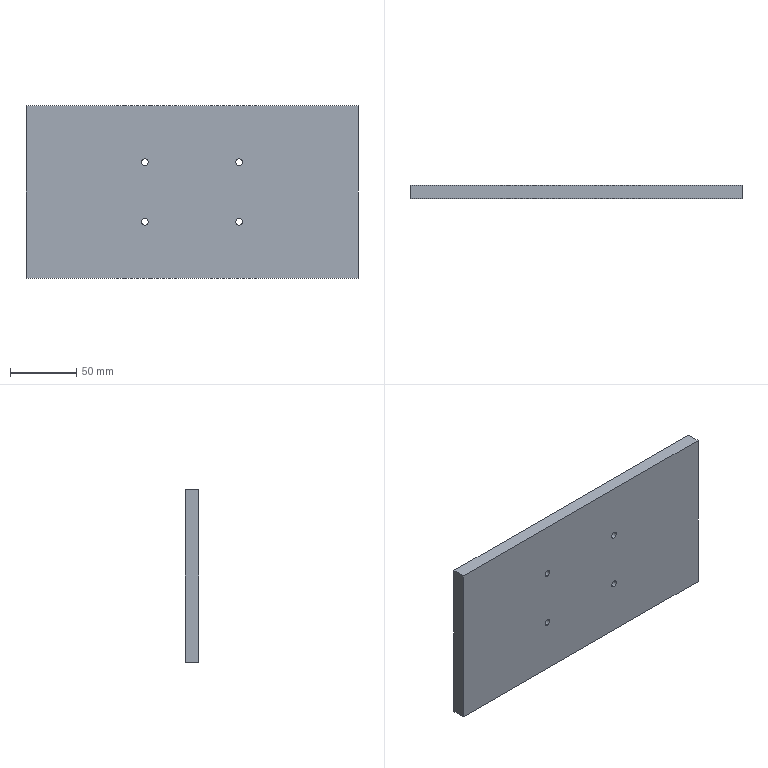Part | STEP file | A14-033 | 1 solid | 22 faces | box 250 x 10 x 130 mm | volume 324205 mm3 | cone 8 | cylinder 8 | plane 6 | commonest cylinder face diameters 5 x8
STEP:
#1=CARTESIAN_POINT('',(0.,0.,0.));
#2=DIRECTION('',(0.,0.,1.));
#3=DIRECTION('',(1.,0.,0.));
#4=AXIS2_PLACEMENT_3D('',#1,#2,#3);
#5=CARTESIAN_POINT('',(35.5,4.475,25.));
#6=VERTEX_POINT('',#5);
#7=CARTESIAN_POINT('',(35.5,5.,25.525));
#8=VERTEX_POINT('',#7);
#9=CARTESIAN_POINT('',(35.5,5.,25.525));
#10=DIRECTION('',(0.,0.7071,0.7071));
#11=VECTOR('',#10,1.);
#12=LINE('',#9,#11);
#13=CARTESIAN_POINT('',(35.5,5.,22.5));
#14=DIRECTION('',(0.,1.,0.));
#15=DIRECTION('',(0.,0.,1.));
#16=AXIS2_PLACEMENT_3D('',#13,#14,#15);
#17=CONICAL_SURFACE('',#16,3.025,0.7854);
#18=CARTESIAN_POINT('',(6.283,0.));
#19=DIRECTION('',(0.,1.));
#20=VECTOR('',#19,1.);
#21=LINE('',#18,#20);
#22=(GEOMETRIC_REPRESENTATION_CONTEXT(2)PARAMETRIC_REPRESENTATION_CONTEXT()REPRESENTATION_CONTEXT('',''));
#23=DEFINITIONAL_REPRESENTATION('',(#21),#22);
#24=PCURVE('',#17,#23);
#25=CARTESIAN_POINT('',(35.5,5.,22.5));
#26=DIRECTION('',(0.,1.,0.));
#27=DIRECTION('',(0.,0.,1.));
#28=AXIS2_PLACEMENT_3D('',#25,#26,#27);
#29=CONICAL_SURFACE('',#28,3.025,0.7854);
#30=CARTESIAN_POINT('',(0.,0.));
#31=DIRECTION('',(0.,1.));
#32=VECTOR('',#31,1.);
#33=LINE('',#30,#32);
#34=(GEOMETRIC_REPRESENTATION_CONTEXT(2)PARAMETRIC_REPRESENTATION_CONTEXT()REPRESENTATION_CONTEXT('',''));
#35=DEFINITIONAL_REPRESENTATION('',(#33),#34);
#36=PCURVE('',#29,#35);
#37=SURFACE_CURVE('',#12,(#24,#36),.PCURVE_S1.);
#38=EDGE_CURVE('',#6,#8,#37,.T.);
#39=ORIENTED_EDGE('',*,*,#38,.T.);
#40=CARTESIAN_POINT('',(35.5,5.,19.475));
#41=VERTEX_POINT('',#40);
#42=CARTESIAN_POINT('',(35.5,5.,22.5));
#43=DIRECTION('',(0.,1.,0.));
#44=DIRECTION('',(0.,0.,1.));
#45=AXIS2_PLACEMENT_3D('',#42,#43,#44);
#46=CIRCLE('',#45,3.025);
#47=CARTESIAN_POINT('',(0.,0.));
#48=DIRECTION('',(1.,0.));
#49=VECTOR('',#48,1.);
#50=LINE('',#47,#49);
#51=(GEOMETRIC_REPRESENTATION_CONTEXT(2)PARAMETRIC_REPRESENTATION_CONTEXT()REPRESENTATION_CONTEXT('',''));
#52=DEFINITIONAL_REPRESENTATION('',(#50),#51);
#53=PCURVE('',#17,#52);
#54=CARTESIAN_POINT('',(0.,5.,0.));
#55=DIRECTION('',(0.,1.,0.));
#56=DIRECTION('',(0.,0.,1.));
#57=AXIS2_PLACEMENT_3D('',#54,#55,#56);
#58=PLANE('',#57);
#59=CARTESIAN_POINT('',(22.5,35.5));
#60=DIRECTION('',(1.,0.));
#61=AXIS2_PLACEMENT_2D('',#59,#60);
#62=CIRCLE('',#61,3.025);
#63=(GEOMETRIC_REPRESENTATION_CONTEXT(2)PARAMETRIC_REPRESENTATION_CONTEXT()REPRESENTATION_CONTEXT('',''));
#64=DEFINITIONAL_REPRESENTATION('',(#62),#63);
#65=PCURVE('',#58,#64);
#66=SURFACE_CURVE('',#46,(#53,#65),.PCURVE_S1.);
#67=EDGE_CURVE('',#41,#8,#66,.T.);
#68=ORIENTED_EDGE('',*,*,#67,.F.);
#69=CARTESIAN_POINT('',(35.5,4.475,20.));
#70=VERTEX_POINT('',#69);
#71=CARTESIAN_POINT('',(35.5,5.,19.475));
#72=DIRECTION('',(0.,0.7071,-0.7071));
#73=VECTOR('',#72,1.);
#74=LINE('',#71,#73);
#75=CARTESIAN_POINT('',(3.142,0.));
#76=DIRECTION('',(0.,1.));
#77=VECTOR('',#76,1.);
#78=LINE('',#75,#77);
#79=(GEOMETRIC_REPRESENTATION_CONTEXT(2)PARAMETRIC_REPRESENTATION_CONTEXT()REPRESENTATION_CONTEXT('',''));
#80=DEFINITIONAL_REPRESENTATION('',(#78),#79);
#81=PCURVE('',#17,#80);
#82=CARTESIAN_POINT('',(3.142,0.));
#83=DIRECTION('',(0.,1.));
#84=VECTOR('',#83,1.);
#85=LINE('',#82,#84);
#86=(GEOMETRIC_REPRESENTATION_CONTEXT(2)PARAMETRIC_REPRESENTATION_CONTEXT()REPRESENTATION_CONTEXT('',''));
#87=DEFINITIONAL_REPRESENTATION('',(#85),#86);
#88=PCURVE('',#29,#87);
#89=SURFACE_CURVE('',#74,(#81,#88),.PCURVE_S1.);
#90=EDGE_CURVE('',#70,#41,#89,.T.);
#91=ORIENTED_EDGE('',*,*,#90,.F.);
#92=CARTESIAN_POINT('',(35.5,4.475,22.5));
#93=DIRECTION('',(0.,1.,0.));
#94=DIRECTION('',(0.,0.,1.));
#95=AXIS2_PLACEMENT_3D('',#92,#93,#94);
#96=CIRCLE('',#95,2.5);
#97=CARTESIAN_POINT('',(0.,-0.525));
#98=DIRECTION('',(1.,0.));
#99=VECTOR('',#98,1.);
#100=LINE('',#97,#99);
#101=(GEOMETRIC_REPRESENTATION_CONTEXT(2)PARAMETRIC_REPRESENTATION_CONTEXT()REPRESENTATION_CONTEXT('',''));
#102=DEFINITIONAL_REPRESENTATION('',(#100),#101);
#103=PCURVE('',#17,#102);
#104=CARTESIAN_POINT('',(35.5,5.,22.5));
#105=DIRECTION('',(0.,1.,0.));
#106=DIRECTION('',(0.,0.,1.));
#107=AXIS2_PLACEMENT_3D('',#104,#105,#106);
#108=CYLINDRICAL_SURFACE('',#107,2.5);
#109=CARTESIAN_POINT('',(0.,-0.525));
#110=DIRECTION('',(1.,0.));
#111=VECTOR('',#110,1.);
#112=LINE('',#109,#111);
#113=(GEOMETRIC_REPRESENTATION_CONTEXT(2)PARAMETRIC_REPRESENTATION_CONTEXT()REPRESENTATION_CONTEXT('',''));
#114=DEFINITIONAL_REPRESENTATION('',(#112),#113);
#115=PCURVE('',#108,#114);
#116=SURFACE_CURVE('',#96,(#103,#115),.PCURVE_S1.);
#117=EDGE_CURVE('',#70,#6,#116,.T.);
#118=ORIENTED_EDGE('',*,*,#117,.T.);
#119=EDGE_LOOP('',(#39,#68,#91,#118));
#120=FACE_BOUND('',#119,.F.);
#121=ADVANCED_FACE('',(#120),#17,.F.);
#122=CARTESIAN_POINT('',(35.5,-5.,25.));
#123=VERTEX_POINT('',#122);
#124=CARTESIAN_POINT('',(35.5,5.,25.));
#125=DIRECTION('',(0.,1.,0.));
#126=VECTOR('',#125,1.);
#127=LINE('',#124,#126);
#128=CARTESIAN_POINT('',(6.283,0.));
#129=DIRECTION('',(0.,1.));
#130=VECTOR('',#129,1.);
#131=LINE('',#128,#130);
#132=(GEOMETRIC_REPRESENTATION_CONTEXT(2)PARAMETRIC_REPRESENTATION_CONTEXT()REPRESENTATION_CONTEXT('',''));
#133=DEFINITIONAL_REPRESENTATION('',(#131),#132);
#134=PCURVE('',#108,#133);
#135=CARTESIAN_POINT('',(35.5,5.,22.5));
#136=DIRECTION('',(0.,1.,0.));
#137=DIRECTION('',(0.,0.,1.));
#138=AXIS2_PLACEMENT_3D('',#135,#136,#137);
#139=CYLINDRICAL_SURFACE('',#138,2.5);
#140=CARTESIAN_POINT('',(0.,0.));
#141=DIRECTION('',(0.,1.));
#142=VECTOR('',#141,1.);
#143=LINE('',#140,#142);
#144=(GEOMETRIC_REPRESENTATION_CONTEXT(2)PARAMETRIC_REPRESENTATION_CONTEXT()REPRESENTATION_CONTEXT('',''));
#145=DEFINITIONAL_REPRESENTATION('',(#143),#144);
#146=PCURVE('',#139,#145);
#147=SURFACE_CURVE('',#127,(#134,#146),.PCURVE_S1.);
#148=EDGE_CURVE('',#123,#6,#147,.T.);
#149=ORIENTED_EDGE('',*,*,#148,.T.);
#150=ORIENTED_EDGE('',*,*,#117,.F.);
#151=CARTESIAN_POINT('',(35.5,-5.,20.));
#152=VERTEX_POINT('',#151);
#153=CARTESIAN_POINT('',(35.5,5.,20.));
#154=DIRECTION('',(0.,1.,0.));
#155=VECTOR('',#154,1.);
#156=LINE('',#153,#155);
#157=CARTESIAN_POINT('',(3.142,0.));
#158=DIRECTION('',(0.,1.));
#159=VECTOR('',#158,1.);
#160=LINE('',#157,#159);
#161=(GEOMETRIC_REPRESENTATION_CONTEXT(2)PARAMETRIC_REPRESENTATION_CONTEXT()REPRESENTATION_CONTEXT('',''));
#162=DEFINITIONAL_REPRESENTATION('',(#160),#161);
#163=PCURVE('',#108,#162);
#164=CARTESIAN_POINT('',(3.142,0.));
#165=DIRECTION('',(0.,1.));
#166=VECTOR('',#165,1.);
#167=LINE('',#164,#166);
#168=(GEOMETRIC_REPRESENTATION_CONTEXT(2)PARAMETRIC_REPRESENTATION_CONTEXT()REPRESENTATION_CONTEXT('',''));
#169=DEFINITIONAL_REPRESENTATION('',(#167),#168);
#170=PCURVE('',#139,#169);
#171=SURFACE_CURVE('',#156,(#163,#170),.PCURVE_S1.);
#172=EDGE_CURVE('',#152,#70,#171,.T.);
#173=ORIENTED_EDGE('',*,*,#172,.F.);
#174=CARTESIAN_POINT('',(35.5,-5.,22.5));
#175=DIRECTION('',(0.,1.,0.));
#176=DIRECTION('',(0.,0.,1.));
#177=AXIS2_PLACEMENT_3D('',#174,#175,#176);
#178=CIRCLE('',#177,2.5);
#179=CARTESIAN_POINT('',(0.,-10.));
#180=DIRECTION('',(1.,0.));
#181=VECTOR('',#180,1.);
#182=LINE('',#179,#181);
#183=(GEOMETRIC_REPRESENTATION_CONTEXT(2)PARAMETRIC_REPRESENTATION_CONTEXT()REPRESENTATION_CONTEXT('',''));
#184=DEFINITIONAL_REPRESENTATION('',(#182),#183);
#185=PCURVE('',#108,#184);
#186=CARTESIAN_POINT('',(0.,-5.,0.));
#187=DIRECTION('',(0.,1.,0.));
#188=DIRECTION('',(0.,0.,1.));
#189=AXIS2_PLACEMENT_3D('',#186,#187,#188);
#190=PLANE('',#189);
#191=CARTESIAN_POINT('',(22.5,35.5));
#192=DIRECTION('',(1.,0.));
#193=AXIS2_PLACEMENT_2D('',#191,#192);
#194=CIRCLE('',#193,2.5);
#195=(GEOMETRIC_REPRESENTATION_CONTEXT(2)PARAMETRIC_REPRESENTATION_CONTEXT()REPRESENTATION_CONTEXT('',''));
#196=DEFINITIONAL_REPRESENTATION('',(#194),#195);
#197=PCURVE('',#190,#196);
#198=SURFACE_CURVE('',#178,(#185,#197),.PCURVE_S1.);
#199=EDGE_CURVE('',#152,#123,#198,.T.);
#200=ORIENTED_EDGE('',*,*,#199,.T.);
#201=EDGE_LOOP('',(#149,#150,#173,#200));
#202=FACE_BOUND('',#201,.F.);
#203=ADVANCED_FACE('',(#202),#108,.F.);
#204=CARTESIAN_POINT('',(35.5,4.475,-20.));
#205=VERTEX_POINT('',#204);
#206=CARTESIAN_POINT('',(35.5,5.,-19.475));
#207=VERTEX_POINT('',#206);
#208=CARTESIAN_POINT('',(35.5,5.,-19.475));
#209=DIRECTION('',(0.,0.7071,0.7071));
#210=VECTOR('',#209,1.);
#211=LINE('',#208,#210);
#212=CARTESIAN_POINT('',(35.5,5.,-22.5));
#213=DIRECTION('',(0.,1.,0.));
#214=DIRECTION('',(0.,0.,1.));
#215=AXIS2_PLACEMENT_3D('',#212,#213,#214);
#216=CONICAL_SURFACE('',#215,3.025,0.7854);
#217=CARTESIAN_POINT('',(6.283,0.));
#218=DIRECTION('',(0.,1.));
#219=VECTOR('',#218,1.);
#220=LINE('',#217,#219);
#221=(GEOMETRIC_REPRESENTATION_CONTEXT(2)PARAMETRIC_REPRESENTATION_CONTEXT()REPRESENTATION_CONTEXT('',''));
#222=DEFINITIONAL_REPRESENTATION('',(#220),#221);
#223=PCURVE('',#216,#222);
#224=CARTESIAN_POINT('',(35.5,5.,-22.5));
#225=DIRECTION('',(0.,1.,0.));
#226=DIRECTION('',(0.,0.,1.));
#227=AXIS2_PLACEMENT_3D('',#224,#225,#226);
#228=CONICAL_SURFACE('',#227,3.025,0.7854);
#229=CARTESIAN_POINT('',(0.,0.));
#230=DIRECTION('',(0.,1.));
#231=VECTOR('',#230,1.);
#232=LINE('',#229,#231);
#233=(GEOMETRIC_REPRESENTATION_CONTEXT(2)PARAMETRIC_REPRESENTATION_CONTEXT()REPRESENTATION_CONTEXT('',''));
#234=DEFINITIONAL_REPRESENTATION('',(#232),#233);
#235=PCURVE('',#228,#234);
#236=SURFACE_CURVE('',#211,(#223,#235),.PCURVE_S1.);
#237=EDGE_CURVE('',#205,#207,#236,.T.);
#238=ORIENTED_EDGE('',*,*,#237,.T.);
#239=CARTESIAN_POINT('',(35.5,5.,-25.525));
#240=VERTEX_POINT('',#239);
#241=CARTESIAN_POINT('',(35.5,5.,-22.5));
#242=DIRECTION('',(0.,1.,0.));
#243=DIRECTION('',(0.,0.,1.));
#244=AXIS2_PLACEMENT_3D('',#241,#242,#243);
#245=CIRCLE('',#244,3.025);
#246=CARTESIAN_POINT('',(0.,0.));
#247=DIRECTION('',(1.,0.));
#248=VECTOR('',#247,1.);
#249=LINE('',#246,#248);
#250=(GEOMETRIC_REPRESENTATION_CONTEXT(2)PARAMETRIC_REPRESENTATION_CONTEXT()REPRESENTATION_CONTEXT('',''));
#251=DEFINITIONAL_REPRESENTATION('',(#249),#250);
#252=PCURVE('',#216,#251);
#253=CARTESIAN_POINT('',(-22.5,35.5));
#254=DIRECTION('',(1.,0.));
#255=AXIS2_PLACEMENT_2D('',#253,#254);
#256=CIRCLE('',#255,3.025);
#257=(GEOMETRIC_REPRESENTATION_CONTEXT(2)PARAMETRIC_REPRESENTATION_CONTEXT()REPRESENTATION_CONTEXT('',''));
#258=DEFINITIONAL_REPRESENTATION('',(#256),#257);
#259=PCURVE('',#58,#258);
#260=SURFACE_CURVE('',#245,(#252,#259),.PCURVE_S1.);
#261=EDGE_CURVE('',#240,#207,#260,.T.);
#262=ORIENTED_EDGE('',*,*,#261,.F.);
#263=CARTESIAN_POINT('',(35.5,4.475,-25.));
#264=VERTEX_POINT('',#263);
#265=CARTESIAN_POINT('',(35.5,5.,-25.525));
#266=DIRECTION('',(0.,0.7071,-0.7071));
#267=VECTOR('',#266,1.);
#268=LINE('',#265,#267);
#269=CARTESIAN_POINT('',(3.142,0.));
#270=DIRECTION('',(0.,1.));
#271=VECTOR('',#270,1.);
#272=LINE('',#269,#271);
#273=(GEOMETRIC_REPRESENTATION_CONTEXT(2)PARAMETRIC_REPRESENTATION_CONTEXT()REPRESENTATION_CONTEXT('',''));
#274=DEFINITIONAL_REPRESENTATION('',(#272),#273);
#275=PCURVE('',#216,#274);
#276=CARTESIAN_POINT('',(3.142,0.));
#277=DIRECTION('',(0.,1.));
#278=VECTOR('',#277,1.);
#279=LINE('',#276,#278);
#280=(GEOMETRIC_REPRESENTATION_CONTEXT(2)PARAMETRIC_REPRESENTATION_CONTEXT()REPRESENTATION_CONTEXT('',''));
#281=DEFINITIONAL_REPRESENTATION('',(#279),#280);
#282=PCURVE('',#228,#281);
#283=SURFACE_CURVE('',#268,(#275,#282),.PCURVE_S1.);
#284=EDGE_CURVE('',#264,#240,#283,.T.);
#285=ORIENTED_EDGE('',*,*,#284,.F.);
#286=CARTESIAN_POINT('',(35.5,4.475,-22.5));
#287=DIRECTION('',(0.,1.,0.));
#288=DIRECTION('',(0.,0.,1.));
#289=AXIS2_PLACEMENT_3D('',#286,#287,#288);
#290=CIRCLE('',#289,2.5);
#291=CARTESIAN_POINT('',(0.,-0.525));
#292=DIRECTION('',(1.,0.));
#293=VECTOR('',#292,1.);
#294=LINE('',#291,#293);
#295=(GEOMETRIC_REPRESENTATION_CONTEXT(2)PARAMETRIC_REPRESENTATION_CONTEXT()REPRESENTATION_CONTEXT('',''));
#296=DEFINITIONAL_REPRESENTATION('',(#294),#295);
#297=PCURVE('',#216,#296);
#298=CARTESIAN_POINT('',(35.5,5.,-22.5));
#299=DIRECTION('',(0.,1.,0.));
#300=DIRECTION('',(0.,0.,1.));
#301=AXIS2_PLACEMENT_3D('',#298,#299,#300);
#302=CYLINDRICAL_SURFACE('',#301,2.5);
#303=CARTESIAN_POINT('',(0.,-0.525));
#304=DIRECTION('',(1.,0.));
#305=VECTOR('',#304,1.);
#306=LINE('',#303,#305);
#307=(GEOMETRIC_REPRESENTATION_CONTEXT(2)PARAMETRIC_REPRESENTATION_CONTEXT()REPRESENTATION_CONTEXT('',''));
#308=DEFINITIONAL_REPRESENTATION('',(#306),#307);
#309=PCURVE('',#302,#308);
#310=SURFACE_CURVE('',#290,(#297,#309),.PCURVE_S1.);
#311=EDGE_CURVE('',#264,#205,#310,.T.);
#312=ORIENTED_EDGE('',*,*,#311,.T.);
#313=EDGE_LOOP('',(#238,#262,#285,#312));
#314=FACE_BOUND('',#313,.F.);
#315=ADVANCED_FACE('',(#314),#216,.F.);
#316=CARTESIAN_POINT('',(35.5,-5.,-20.));
#317=VERTEX_POINT('',#316);
#318=CARTESIAN_POINT('',(35.5,5.,-20.));
#319=DIRECTION('',(0.,1.,0.));
#320=VECTOR('',#319,1.);
#321=LINE('',#318,#320);
#322=CARTESIAN_POINT('',(6.283,0.));
#323=DIRECTION('',(0.,1.));
#324=VECTOR('',#323,1.);
#325=LINE('',#322,#324);
#326=(GEOMETRIC_REPRESENTATION_CONTEXT(2)PARAMETRIC_REPRESENTATION_CONTEXT()REPRESENTATION_CONTEXT('',''));
#327=DEFINITIONAL_REPRESENTATION('',(#325),#326);
#328=PCURVE('',#302,#327);
#329=CARTESIAN_POINT('',(35.5,5.,-22.5));
#330=DIRECTION('',(0.,1.,0.));
#331=DIRECTION('',(0.,0.,1.));
#332=AXIS2_PLACEMENT_3D('',#329,#330,#331);
#333=CYLINDRICAL_SURFACE('',#332,2.5);
#334=CARTESIAN_POINT('',(0.,0.));
#335=DIRECTION('',(0.,1.));
#336=VECTOR('',#335,1.);
#337=LINE('',#334,#336);
#338=(GEOMETRIC_REPRESENTATION_CONTEXT(2)PARAMETRIC_REPRESENTATION_CONTEXT()REPRESENTATION_CONTEXT('',''));
#339=DEFINITIONAL_REPRESENTATION('',(#337),#338);
#340=PCURVE('',#333,#339);
#341=SURFACE_CURVE('',#321,(#328,#340),.PCURVE_S1.);
#342=EDGE_CURVE('',#317,#205,#341,.T.);
#343=ORIENTED_EDGE('',*,*,#342,.T.);
#344=ORIENTED_EDGE('',*,*,#311,.F.);
#345=CARTESIAN_POINT('',(35.5,-5.,-25.));
#346=VERTEX_POINT('',#345);
#347=CARTESIAN_POINT('',(35.5,5.,-25.));
#348=DIRECTION('',(0.,1.,0.));
#349=VECTOR('',#348,1.);
#350=LINE('',#347,#349);
#351=CARTESIAN_POINT('',(3.142,0.));
#352=DIRECTION('',(0.,1.));
#353=VECTOR('',#352,1.);
#354=LINE('',#351,#353);
#355=(GEOMETRIC_REPRESENTATION_CONTEXT(2)PARAMETRIC_REPRESENTATION_CONTEXT()REPRESENTATION_CONTEXT('',''));
#356=DEFINITIONAL_REPRESENTATION('',(#354),#355);
#357=PCURVE('',#302,#356);
#358=CARTESIAN_POINT('',(3.142,0.));
#359=DIRECTION('',(0.,1.));
#360=VECTOR('',#359,1.);
#361=LINE('',#358,#360);
#362=(GEOMETRIC_REPRESENTATION_CONTEXT(2)PARAMETRIC_REPRESENTATION_CONTEXT()REPRESENTATION_CONTEXT('',''));
#363=DEFINITIONAL_REPRESENTATION('',(#361),#362);
#364=PCURVE('',#333,#363);
#365=SURFACE_CURVE('',#350,(#357,#364),.PCURVE_S1.);
#366=EDGE_CURVE('',#346,#264,#365,.T.);
#367=ORIENTED_EDGE('',*,*,#366,.F.);
#368=CARTESIAN_POINT('',(35.5,-5.,-22.5));
#369=DIRECTION('',(0.,1.,0.));
#370=DIRECTION('',(0.,0.,1.));
#371=AXIS2_PLACEMENT_3D('',#368,#369,#370);
#372=CIRCLE('',#371,2.5);
#373=CARTESIAN_POINT('',(0.,-10.));
#374=DIRECTION('',(1.,0.));
#375=VECTOR('',#374,1.);
#376=LINE('',#373,#375);
#377=(GEOMETRIC_REPRESENTATION_CONTEXT(2)PARAMETRIC_REPRESENTATION_CONTEXT()REPRESENTATION_CONTEXT('',''));
#378=DEFINITIONAL_REPRESENTATION('',(#376),#377);
#379=PCURVE('',#302,#378);
#380=CARTESIAN_POINT('',(-22.5,35.5));
#381=DIRECTION('',(1.,0.));
#382=AXIS2_PLACEMENT_2D('',#380,#381);
#383=CIRCLE('',#382,2.5);
#384=(GEOMETRIC_REPRESENTATION_CONTEXT(2)PARAMETRIC_REPRESENTATION_CONTEXT()REPRESENTATION_CONTEXT('',''));
#385=DEFINITIONAL_REPRESENTATION('',(#383),#384);
#386=PCURVE('',#190,#385);
#387=SURFACE_CURVE('',#372,(#379,#386),.PCURVE_S1.);
#388=EDGE_CURVE('',#346,#317,#387,.T.);
#389=ORIENTED_EDGE('',*,*,#388,.T.);
#390=EDGE_LOOP('',(#343,#344,#367,#389));
#391=FACE_BOUND('',#390,.F.);
#392=ADVANCED_FACE('',(#391),#302,.F.);
#393=CARTESIAN_POINT('',(-35.5,4.475,25.));
#394=VERTEX_POINT('',#393);
#395=CARTESIAN_POINT('',(-35.5,5.,25.525));
#396=VERTEX_POINT('',#395);
#397=CARTESIAN_POINT('',(-35.5,5.,25.525));
#398=DIRECTION('',(0.,0.7071,0.7071));
#399=VECTOR('',#398,1.);
#400=LINE('',#397,#399);
#401=CARTESIAN_POINT('',(-35.5,5.,22.5));
#402=DIRECTION('',(0.,1.,0.));
#403=DIRECTION('',(0.,0.,1.));
#404=AXIS2_PLACEMENT_3D('',#401,#402,#403);
#405=CONICAL_SURFACE('',#404,3.025,0.7854);
#406=CARTESIAN_POINT('',(6.283,0.));
#407=DIRECTION('',(0.,1.));
#408=VECTOR('',#407,1.);
#409=LINE('',#406,#408);
#410=(GEOMETRIC_REPRESENTATION_CONTEXT(2)PARAMETRIC_REPRESENTATION_CONTEXT()REPRESENTATION_CONTEXT('',''));
#411=DEFINITIONAL_REPRESENTATION('',(#409),#410);
#412=PCURVE('',#405,#411);
#413=CARTESIAN_POINT('',(-35.5,5.,22.5));
#414=DIRECTION('',(0.,1.,0.));
#415=DIRECTION('',(0.,0.,1.));
#416=AXIS2_PLACEMENT_3D('',#413,#414,#415);
#417=CONICAL_SURFACE('',#416,3.025,0.7854);
#418=CARTESIAN_POINT('',(0.,0.));
#419=DIRECTION('',(0.,1.));
#420=VECTOR('',#419,1.);
#421=LINE('',#418,#420);
#422=(GEOMETRIC_REPRESENTATION_CONTEXT(2)PARAMETRIC_REPRESENTATION_CONTEXT()REPRESENTATION_CONTEXT('',''));
#423=DEFINITIONAL_REPRESENTATION('',(#421),#422);
#424=PCURVE('',#417,#423);
#425=SURFACE_CURVE('',#400,(#412,#424),.PCURVE_S1.);
#426=EDGE_CURVE('',#394,#396,#425,.T.);
#427=ORIENTED_EDGE('',*,*,#426,.T.);
#428=CARTESIAN_POINT('',(-35.5,5.,19.475));
#429=VERTEX_POINT('',#428);
#430=CARTESIAN_POINT('',(-35.5,5.,22.5));
#431=DIRECTION('',(0.,1.,0.));
#432=DIRECTION('',(0.,0.,1.));
#433=AXIS2_PLACEMENT_3D('',#430,#431,#432);
#434=CIRCLE('',#433,3.025);
#435=CARTESIAN_POINT('',(0.,0.));
#436=DIRECTION('',(1.,0.));
#437=VECTOR('',#436,1.);
#438=LINE('',#435,#437);
#439=(GEOMETRIC_REPRESENTATION_CONTEXT(2)PARAMETRIC_REPRESENTATION_CONTEXT()REPRESENTATION_CONTEXT('',''));
#440=DEFINITIONAL_REPRESENTATION('',(#438),#439);
#441=PCURVE('',#405,#440);
#442=CARTESIAN_POINT('',(22.5,-35.5));
#443=DIRECTION('',(1.,0.));
#444=AXIS2_PLACEMENT_2D('',#442,#443);
#445=CIRCLE('',#444,3.025);
#446=(GEOMETRIC_REPRESENTATION_CONTEXT(2)PARAMETRIC_REPRESENTATION_CONTEXT()REPRESENTATION_CONTEXT('',''));
#447=DEFINITIONAL_REPRESENTATION('',(#445),#446);
#448=PCURVE('',#58,#447);
#449=SURFACE_CURVE('',#434,(#441,#448),.PCURVE_S1.);
#450=EDGE_CURVE('',#429,#396,#449,.T.);
#451=ORIENTED_EDGE('',*,*,#450,.F.);
#452=CARTESIAN_POINT('',(-35.5,4.475,20.));
#453=VERTEX_POINT('',#452);
#454=CARTESIAN_POINT('',(-35.5,5.,19.475));
#455=DIRECTION('',(0.,0.7071,-0.7071));
#456=VECTOR('',#455,1.);
#457=LINE('',#454,#456);
#458=CARTESIAN_POINT('',(3.142,0.));
#459=DIRECTION('',(0.,1.));
#460=VECTOR('',#459,1.);
#461=LINE('',#458,#460);
#462=(GEOMETRIC_REPRESENTATION_CONTEXT(2)PARAMETRIC_REPRESENTATION_CONTEXT()REPRESENTATION_CONTEXT('',''));
#463=DEFINITIONAL_REPRESENTATION('',(#461),#462);
#464=PCURVE('',#405,#463);
#465=CARTESIAN_POINT('',(3.142,0.));
#466=DIRECTION('',(0.,1.));
#467=VECTOR('',#466,1.);
#468=LINE('',#465,#467);
#469=(GEOMETRIC_REPRESENTATION_CONTEXT(2)PARAMETRIC_REPRESENTATION_CONTEXT()REPRESENTATION_CONTEXT('',''));
#470=DEFINITIONAL_REPRESENTATION('',(#468),#469);
#471=PCURVE('',#417,#470);
#472=SURFACE_CURVE('',#457,(#464,#471),.PCURVE_S1.);
#473=EDGE_CURVE('',#453,#429,#472,.T.);
#474=ORIENTED_EDGE('',*,*,#473,.F.);
#475=CARTESIAN_POINT('',(-35.5,4.475,22.5));
#476=DIRECTION('',(0.,1.,0.));
#477=DIRECTION('',(0.,0.,1.));
#478=AXIS2_PLACEMENT_3D('',#475,#476,#477);
#479=CIRCLE('',#478,2.5);
#480=CARTESIAN_POINT('',(0.,-0.525));
#481=DIRECTION('',(1.,0.));
#482=VECTOR('',#481,1.);
#483=LINE('',#480,#482);
#484=(GEOMETRIC_REPRESENTATION_CONTEXT(2)PARAMETRIC_REPRESENTATION_CONTEXT()REPRESENTATION_CONTEXT('',''));
#485=DEFINITIONAL_REPRESENTATION('',(#483),#484);
#486=PCURVE('',#405,#485);
#487=CARTESIAN_POINT('',(-35.5,5.,22.5));
#488=DIRECTION('',(0.,1.,0.));
#489=DIRECTION('',(0.,0.,1.));
#490=AXIS2_PLACEMENT_3D('',#487,#488,#489);
#491=CYLINDRICAL_SURFACE('',#490,2.5);
#492=CARTESIAN_POINT('',(0.,-0.525));
#493=DIRECTION('',(1.,0.));
#494=VECTOR('',#493,1.);
#495=LINE('',#492,#494);
#496=(GEOMETRIC_REPRESENTATION_CONTEXT(2)PARAMETRIC_REPRESENTATION_CONTEXT()REPRESENTATION_CONTEXT('',''));
#497=DEFINITIONAL_REPRESENTATION('',(#495),#496);
#498=PCURVE('',#491,#497);
#499=SURFACE_CURVE('',#479,(#486,#498),.PCURVE_S1.);
#500=EDGE_CURVE('',#453,#394,#499,.T.);
#501=ORIENTED_EDGE('',*,*,#500,.T.);
#502=EDGE_LOOP('',(#427,#451,#474,#501));
#503=FACE_BOUND('',#502,.F.);
#504=ADVANCED_FACE('',(#503),#405,.F.);
#505=CARTESIAN_POINT('',(-35.5,-5.,25.));
#506=VERTEX_POINT('',#505);
#507=CARTESIAN_POINT('',(-35.5,5.,25.));
#508=DIRECTION('',(0.,1.,0.));
#509=VECTOR('',#508,1.);
#510=LINE('',#507,#509);
#511=CARTESIAN_POINT('',(6.283,0.));
#512=DIRECTION('',(0.,1.));
#513=VECTOR('',#512,1.);
#514=LINE('',#511,#513);
#515=(GEOMETRIC_REPRESENTATION_CONTEXT(2)PARAMETRIC_REPRESENTATION_CONTEXT()REPRESENTATION_CONTEXT('',''));
#516=DEFINITIONAL_REPRESENTATION('',(#514),#515);
#517=PCURVE('',#491,#516);
#518=CARTESIAN_POINT('',(-35.5,5.,22.5));
#519=DIRECTION('',(0.,1.,0.));
#520=DIRECTION('',(0.,0.,1.));
#521=AXIS2_PLACEMENT_3D('',#518,#519,#520);
#522=CYLINDRICAL_SURFACE('',#521,2.5);
#523=CARTESIAN_POINT('',(0.,0.));
#524=DIRECTION('',(0.,1.));
#525=VECTOR('',#524,1.);
#526=LINE('',#523,#525);
#527=(GEOMETRIC_REPRESENTATION_CONTEXT(2)PARAMETRIC_REPRESENTATION_CONTEXT()REPRESENTATION_CONTEXT('',''));
#528=DEFINITIONAL_REPRESENTATION('',(#526),#527);
#529=PCURVE('',#522,#528);
#530=SURFACE_CURVE('',#510,(#517,#529),.PCURVE_S1.);
#531=EDGE_CURVE('',#506,#394,#530,.T.);
#532=ORIENTED_EDGE('',*,*,#531,.T.);
#533=ORIENTED_EDGE('',*,*,#500,.F.);
#534=CARTESIAN_POINT('',(-35.5,-5.,20.));
#535=VERTEX_POINT('',#534);
#536=CARTESIAN_POINT('',(-35.5,5.,20.));
#537=DIRECTION('',(0.,1.,0.));
#538=VECTOR('',#537,1.);
#539=LINE('',#536,#538);
#540=CARTESIAN_POINT('',(3.142,0.));
#541=DIRECTION('',(0.,1.));
#542=VECTOR('',#541,1.);
#543=LINE('',#540,#542);
#544=(GEOMETRIC_REPRESENTATION_CONTEXT(2)PARAMETRIC_REPRESENTATION_CONTEXT()REPRESENTATION_CONTEXT('',''));
#545=DEFINITIONAL_REPRESENTATION('',(#543),#544);
#546=PCURVE('',#491,#545);
#547=CARTESIAN_POINT('',(3.142,0.));
#548=DIRECTION('',(0.,1.));
#549=VECTOR('',#548,1.);
#550=LINE('',#547,#549);
#551=(GEOMETRIC_REPRESENTATION_CONTEXT(2)PARAMETRIC_REPRESENTATION_CONTEXT()REPRESENTATION_CONTEXT('',''));
#552=DEFINITIONAL_REPRESENTATION('',(#550),#551);
#553=PCURVE('',#522,#552);
#554=SURFACE_CURVE('',#539,(#546,#553),.PCURVE_S1.);
#555=EDGE_CURVE('',#535,#453,#554,.T.);
#556=ORIENTED_EDGE('',*,*,#555,.F.);
#557=CARTESIAN_POINT('',(-35.5,-5.,22.5));
#558=DIRECTION('',(0.,1.,0.));
#559=DIRECTION('',(0.,0.,1.));
#560=AXIS2_PLACEMENT_3D('',#557,#558,#559);
#561=CIRCLE('',#560,2.5);
#562=CARTESIAN_POINT('',(0.,-10.));
#563=DIRECTION('',(1.,0.));
#564=VECTOR('',#563,1.);
#565=LINE('',#562,#564);
#566=(GEOMETRIC_REPRESENTATION_CONTEXT(2)PARAMETRIC_REPRESENTATION_CONTEXT()REPRESENTATION_CONTEXT('',''));
#567=DEFINITIONAL_REPRESENTATION('',(#565),#566);
#568=PCURVE('',#491,#567);
#569=CARTESIAN_POINT('',(22.5,-35.5));
#570=DIRECTION('',(1.,0.));
#571=AXIS2_PLACEMENT_2D('',#569,#570);
#572=CIRCLE('',#571,2.5);
#573=(GEOMETRIC_REPRESENTATION_CONTEXT(2)PARAMETRIC_REPRESENTATION_CONTEXT()REPRESENTATION_CONTEXT('',''));
#574=DEFINITIONAL_REPRESENTATION('',(#572),#573);
#575=PCURVE('',#190,#574);
#576=SURFACE_CURVE('',#561,(#568,#575),.PCURVE_S1.);
#577=EDGE_CURVE('',#535,#506,#576,.T.);
#578=ORIENTED_EDGE('',*,*,#577,.T.);
#579=EDGE_LOOP('',(#532,#533,#556,#578));
#580=FACE_BOUND('',#579,.F.);
#581=ADVANCED_FACE('',(#580),#491,.F.);
#582=CARTESIAN_POINT('',(-35.5,4.475,-20.));
#583=VERTEX_POINT('',#582);
#584=CARTESIAN_POINT('',(-35.5,5.,-19.475));
#585=VERTEX_POINT('',#584);
#586=CARTESIAN_POINT('',(-35.5,5.,-19.475));
#587=DIRECTION('',(0.,0.7071,0.7071));
#588=VECTOR('',#587,1.);
#589=LINE('',#586,#588);
#590=CARTESIAN_POINT('',(-35.5,5.,-22.5));
#591=DIRECTION('',(0.,1.,0.));
#592=DIRECTION('',(0.,0.,1.));
#593=AXIS2_PLACEMENT_3D('',#590,#591,#592);
#594=CONICAL_SURFACE('',#593,3.025,0.7854);
#595=CARTESIAN_POINT('',(6.283,0.));
#596=DIRECTION('',(0.,1.));
#597=VECTOR('',#596,1.);
#598=LINE('',#595,#597);
#599=(GEOMETRIC_REPRESENTATION_CONTEXT(2)PARAMETRIC_REPRESENTATION_CONTEXT()REPRESENTATION_CONTEXT('',''));
#600=DEFINITIONAL_REPRESENTATION('',(#598),#599);
#601=PCURVE('',#594,#600);
#602=CARTESIAN_POINT('',(-35.5,5.,-22.5));
#603=DIRECTION('',(0.,1.,0.));
#604=DIRECTION('',(0.,0.,1.));
#605=AXIS2_PLACEMENT_3D('',#602,#603,#604);
#606=CONICAL_SURFACE('',#605,3.025,0.7854);
#607=CARTESIAN_POINT('',(0.,0.));
#608=DIRECTION('',(0.,1.));
#609=VECTOR('',#608,1.);
#610=LINE('',#607,#609);
#611=(GEOMETRIC_REPRESENTATION_CONTEXT(2)PARAMETRIC_REPRESENTATION_CONTEXT()REPRESENTATION_CONTEXT('',''));
#612=DEFINITIONAL_REPRESENTATION('',(#610),#611);
#613=PCURVE('',#606,#612);
#614=SURFACE_CURVE('',#589,(#601,#613),.PCURVE_S1.);
#615=EDGE_CURVE('',#583,#585,#614,.T.);
#616=ORIENTED_EDGE('',*,*,#615,.T.);
#617=CARTESIAN_POINT('',(-35.5,5.,-25.525));
#618=VERTEX_POINT('',#617);
#619=CARTESIAN_POINT('',(-35.5,5.,-22.5));
#620=DIRECTION('',(0.,1.,0.));
#621=DIRECTION('',(0.,0.,1.));
#622=AXIS2_PLACEMENT_3D('',#619,#620,#621);
#623=CIRCLE('',#622,3.025);
#624=CARTESIAN_POINT('',(0.,0.));
#625=DIRECTION('',(1.,0.));
#626=VECTOR('',#625,1.);
#627=LINE('',#624,#626);
#628=(GEOMETRIC_REPRESENTATION_CONTEXT(2)PARAMETRIC_REPRESENTATION_CONTEXT()REPRESENTATION_CONTEXT('',''));
#629=DEFINITIONAL_REPRESENTATION('',(#627),#628);
#630=PCURVE('',#594,#629);
#631=CARTESIAN_POINT('',(-22.5,-35.5));
#632=DIRECTION('',(1.,0.));
#633=AXIS2_PLACEMENT_2D('',#631,#632);
#634=CIRCLE('',#633,3.025);
#635=(GEOMETRIC_REPRESENTATION_CONTEXT(2)PARAMETRIC_REPRESENTATION_CONTEXT()REPRESENTATION_CONTEXT('',''));
#636=DEFINITIONAL_REPRESENTATION('',(#634),#635);
#637=PCURVE('',#58,#636);
#638=SURFACE_CURVE('',#623,(#630,#637),.PCURVE_S1.);
#639=EDGE_CURVE('',#618,#585,#638,.T.);
#640=ORIENTED_EDGE('',*,*,#639,.F.);
#641=CARTESIAN_POINT('',(-35.5,4.475,-25.));
#642=VERTEX_POINT('',#641);
#643=CARTESIAN_POINT('',(-35.5,5.,-25.525));
#644=DIRECTION('',(0.,0.7071,-0.7071));
#645=VECTOR('',#644,1.);
#646=LINE('',#643,#645);
#647=CARTESIAN_POINT('',(3.142,0.));
#648=DIRECTION('',(0.,1.));
#649=VECTOR('',#648,1.);
#650=LINE('',#647,#649);
#651=(GEOMETRIC_REPRESENTATION_CONTEXT(2)PARAMETRIC_REPRESENTATION_CONTEXT()REPRESENTATION_CONTEXT('',''));
#652=DEFINITIONAL_REPRESENTATION('',(#650),#651);
#653=PCURVE('',#594,#652);
#654=CARTESIAN_POINT('',(3.142,0.));
#655=DIRECTION('',(0.,1.));
#656=VECTOR('',#655,1.);
#657=LINE('',#654,#656);
#658=(GEOMETRIC_REPRESENTATION_CONTEXT(2)PARAMETRIC_REPRESENTATION_CONTEXT()REPRESENTATION_CONTEXT('',''));
#659=DEFINITIONAL_REPRESENTATION('',(#657),#658);
#660=PCURVE('',#606,#659);
#661=SURFACE_CURVE('',#646,(#653,#660),.PCURVE_S1.);
#662=EDGE_CURVE('',#642,#618,#661,.T.);
#663=ORIENTED_EDGE('',*,*,#662,.F.);
#664=CARTESIAN_POINT('',(-35.5,4.475,-22.5));
#665=DIRECTION('',(0.,1.,0.));
#666=DIRECTION('',(0.,0.,1.));
#667=AXIS2_PLACEMENT_3D('',#664,#665,#666);
#668=CIRCLE('',#667,2.5);
#669=CARTESIAN_POINT('',(0.,-0.525));
#670=DIRECTION('',(1.,0.));
#671=VECTOR('',#670,1.);
#672=LINE('',#669,#671);
#673=(GEOMETRIC_REPRESENTATION_CONTEXT(2)PARAMETRIC_REPRESENTATION_CONTEXT()REPRESENTATION_CONTEXT('',''));
#674=DEFINITIONAL_REPRESENTATION('',(#672),#673);
#675=PCURVE('',#594,#674);
#676=CARTESIAN_POINT('',(-35.5,5.,-22.5));
#677=DIRECTION('',(0.,1.,0.));
#678=DIRECTION('',(0.,0.,1.));
#679=AXIS2_PLACEMENT_3D('',#676,#677,#678);
#680=CYLINDRICAL_SURFACE('',#679,2.5);
#681=CARTESIAN_POINT('',(0.,-0.525));
#682=DIRECTION('',(1.,0.));
#683=VECTOR('',#682,1.);
#684=LINE('',#681,#683);
#685=(GEOMETRIC_REPRESENTATION_CONTEXT(2)PARAMETRIC_REPRESENTATION_CONTEXT()REPRESENTATION_CONTEXT('',''));
#686=DEFINITIONAL_REPRESENTATION('',(#684),#685);
#687=PCURVE('',#680,#686);
#688=SURFACE_CURVE('',#668,(#675,#687),.PCURVE_S1.);
#689=EDGE_CURVE('',#642,#583,#688,.T.);
#690=ORIENTED_EDGE('',*,*,#689,.T.);
#691=EDGE_LOOP('',(#616,#640,#663,#690));
#692=FACE_BOUND('',#691,.F.);
#693=ADVANCED_FACE('',(#692),#594,.F.);
#694=CARTESIAN_POINT('',(-35.5,-5.,-20.));
#695=VERTEX_POINT('',#694);
#696=CARTESIAN_POINT('',(-35.5,5.,-20.));
#697=DIRECTION('',(0.,1.,0.));
#698=VECTOR('',#697,1.);
#699=LINE('',#696,#698);
#700=CARTESIAN_POINT('',(6.283,0.));
#701=DIRECTION('',(0.,1.));
#702=VECTOR('',#701,1.);
#703=LINE('',#700,#702);
#704=(GEOMETRIC_REPRESENTATION_CONTEXT(2)PARAMETRIC_REPRESENTATION_CONTEXT()REPRESENTATION_CONTEXT('',''));
#705=DEFINITIONAL_REPRESENTATION('',(#703),#704);
#706=PCURVE('',#680,#705);
#707=CARTESIAN_POINT('',(-35.5,5.,-22.5));
#708=DIRECTION('',(0.,1.,0.));
#709=DIRECTION('',(0.,0.,1.));
#710=AXIS2_PLACEMENT_3D('',#707,#708,#709);
#711=CYLINDRICAL_SURFACE('',#710,2.5);
#712=CARTESIAN_POINT('',(0.,0.));
#713=DIRECTION('',(0.,1.));
#714=VECTOR('',#713,1.);
#715=LINE('',#712,#714);
#716=(GEOMETRIC_REPRESENTATION_CONTEXT(2)PARAMETRIC_REPRESENTATION_CONTEXT()REPRESENTATION_CONTEXT('',''));
#717=DEFINITIONAL_REPRESENTATION('',(#715),#716);
#718=PCURVE('',#711,#717);
#719=SURFACE_CURVE('',#699,(#706,#718),.PCURVE_S1.);
#720=EDGE_CURVE('',#695,#583,#719,.T.);
#721=ORIENTED_EDGE('',*,*,#720,.T.);
#722=ORIENTED_EDGE('',*,*,#689,.F.);
#723=CARTESIAN_POINT('',(-35.5,-5.,-25.));
#724=VERTEX_POINT('',#723);
#725=CARTESIAN_POINT('',(-35.5,5.,-25.));
#726=DIRECTION('',(0.,1.,0.));
#727=VECTOR('',#726,1.);
#728=LINE('',#725,#727);
#729=CARTESIAN_POINT('',(3.142,0.));
#730=DIRECTION('',(0.,1.));
#731=VECTOR('',#730,1.);
#732=LINE('',#729,#731);
#733=(GEOMETRIC_REPRESENTATION_CONTEXT(2)PARAMETRIC_REPRESENTATION_CONTEXT()REPRESENTATION_CONTEXT('',''));
#734=DEFINITIONAL_REPRESENTATION('',(#732),#733);
#735=PCURVE('',#680,#734);
#736=CARTESIAN_POINT('',(3.142,0.));
#737=DIRECTION('',(0.,1.));
#738=VECTOR('',#737,1.);
#739=LINE('',#736,#738);
#740=(GEOMETRIC_REPRESENTATION_CONTEXT(2)PARAMETRIC_REPRESENTATION_CONTEXT()REPRESENTATION_CONTEXT('',''));
#741=DEFINITIONAL_REPRESENTATION('',(#739),#740);
#742=PCURVE('',#711,#741);
#743=SURFACE_CURVE('',#728,(#735,#742),.PCURVE_S1.);
#744=EDGE_CURVE('',#724,#642,#743,.T.);
#745=ORIENTED_EDGE('',*,*,#744,.F.);
#746=CARTESIAN_POINT('',(-35.5,-5.,-22.5));
#747=DIRECTION('',(0.,1.,0.));
#748=DIRECTION('',(0.,0.,1.));
#749=AXIS2_PLACEMENT_3D('',#746,#747,#748);
#750=CIRCLE('',#749,2.5);
#751=CARTESIAN_POINT('',(0.,-10.));
#752=DIRECTION('',(1.,0.));
#753=VECTOR('',#752,1.);
#754=LINE('',#751,#753);
#755=(GEOMETRIC_REPRESENTATION_CONTEXT(2)PARAMETRIC_REPRESENTATION_CONTEXT()REPRESENTATION_CONTEXT('',''));
#756=DEFINITIONAL_REPRESENTATION('',(#754),#755);
#757=PCURVE('',#680,#756);
#758=CARTESIAN_POINT('',(-22.5,-35.5));
#759=DIRECTION('',(1.,0.));
#760=AXIS2_PLACEMENT_2D('',#758,#759);
#761=CIRCLE('',#760,2.5);
#762=(GEOMETRIC_REPRESENTATION_CONTEXT(2)PARAMETRIC_REPRESENTATION_CONTEXT()REPRESENTATION_CONTEXT('',''));
#763=DEFINITIONAL_REPRESENTATION('',(#761),#762);
#764=PCURVE('',#190,#763);
#765=SURFACE_CURVE('',#750,(#757,#764),.PCURVE_S1.);
#766=EDGE_CURVE('',#724,#695,#765,.T.);
#767=ORIENTED_EDGE('',*,*,#766,.T.);
#768=EDGE_LOOP('',(#721,#722,#745,#767));
#769=FACE_BOUND('',#768,.F.);
#770=ADVANCED_FACE('',(#769),#680,.F.);
#771=CARTESIAN_POINT('',(125.,-5.,65.));
#772=VERTEX_POINT('',#771);
#773=CARTESIAN_POINT('',(125.,-5.,-65.));
#774=VERTEX_POINT('',#773);
#775=CARTESIAN_POINT('',(125.,-5.,-65.));
#776=DIRECTION('',(0.,0.,-1.));
#777=VECTOR('',#776,1.);
#778=LINE('',#775,#777);
#779=CARTESIAN_POINT('',(125.,5.,-65.));
#780=DIRECTION('',(-1.,0.,0.));
#781=DIRECTION('',(0.,0.,1.));
#782=AXIS2_PLACEMENT_3D('',#779,#780,#781);
#783=PLANE('',#782);
#784=CARTESIAN_POINT('',(0.,-10.));
#785=DIRECTION('',(-1.,0.));
#786=VECTOR('',#785,1.);
#787=LINE('',#784,#786);
#788=(GEOMETRIC_REPRESENTATION_CONTEXT(2)PARAMETRIC_REPRESENTATION_CONTEXT()REPRESENTATION_CONTEXT('',''));
#789=DEFINITIONAL_REPRESENTATION('',(#787),#788);
#790=PCURVE('',#783,#789);
#791=CARTESIAN_POINT('',(-65.,125.));
#792=DIRECTION('',(-1.,0.));
#793=VECTOR('',#792,1.);
#794=LINE('',#791,#793);
#795=(GEOMETRIC_REPRESENTATION_CONTEXT(2)PARAMETRIC_REPRESENTATION_CONTEXT()REPRESENTATION_CONTEXT('',''));
#796=DEFINITIONAL_REPRESENTATION('',(#794),#795);
#797=PCURVE('',#190,#796);
#798=SURFACE_CURVE('',#778,(#790,#797),.PCURVE_S1.);
#799=EDGE_CURVE('',#772,#774,#798,.T.);
#800=ORIENTED_EDGE('',*,*,#799,.T.);
#801=CARTESIAN_POINT('',(125.,5.,-65.));
#802=VERTEX_POINT('',#801);
#803=CARTESIAN_POINT('',(125.,5.,-65.));
#804=DIRECTION('',(0.,-1.,0.));
#805=VECTOR('',#804,1.);
#806=LINE('',#803,#805);
#807=CARTESIAN_POINT('',(0.,0.));
#808=DIRECTION('',(0.,-1.));
#809=VECTOR('',#808,1.);
#810=LINE('',#807,#809);
#811=(GEOMETRIC_REPRESENTATION_CONTEXT(2)PARAMETRIC_REPRESENTATION_CONTEXT()REPRESENTATION_CONTEXT('',''));
#812=DEFINITIONAL_REPRESENTATION('',(#810),#811);
#813=PCURVE('',#783,#812);
#814=CARTESIAN_POINT('',(-125.,5.,-65.));
#815=DIRECTION('',(0.,0.,1.));
#816=DIRECTION('',(1.,0.,0.));
#817=AXIS2_PLACEMENT_3D('',#814,#815,#816);
#818=PLANE('',#817);
#819=CARTESIAN_POINT('',(250.,0.));
#820=DIRECTION('',(0.,-1.));
#821=VECTOR('',#820,1.);
#822=LINE('',#819,#821);
#823=(GEOMETRIC_REPRESENTATION_CONTEXT(2)PARAMETRIC_REPRESENTATION_CONTEXT()REPRESENTATION_CONTEXT('',''));
#824=DEFINITIONAL_REPRESENTATION('',(#822),#823);
#825=PCURVE('',#818,#824);
#826=SURFACE_CURVE('',#806,(#813,#825),.PCURVE_S1.);
#827=EDGE_CURVE('',#802,#774,#826,.T.);
#828=ORIENTED_EDGE('',*,*,#827,.F.);
#829=CARTESIAN_POINT('',(125.,5.,65.));
#830=VERTEX_POINT('',#829);
#831=CARTESIAN_POINT('',(125.,5.,-65.));
#832=DIRECTION('',(0.,0.,-1.));
#833=VECTOR('',#832,1.);
#834=LINE('',#831,#833);
#835=CARTESIAN_POINT('',(0.,0.));
#836=DIRECTION('',(-1.,0.));
#837=VECTOR('',#836,1.);
#838=LINE('',#835,#837);
#839=(GEOMETRIC_REPRESENTATION_CONTEXT(2)PARAMETRIC_REPRESENTATION_CONTEXT()REPRESENTATION_CONTEXT('',''));
#840=DEFINITIONAL_REPRESENTATION('',(#838),#839);
#841=PCURVE('',#783,#840);
#842=CARTESIAN_POINT('',(-65.,125.));
#843=DIRECTION('',(-1.,0.));
#844=VECTOR('',#843,1.);
#845=LINE('',#842,#844);
#846=(GEOMETRIC_REPRESENTATION_CONTEXT(2)PARAMETRIC_REPRESENTATION_CONTEXT()REPRESENTATION_CONTEXT('',''));
#847=DEFINITIONAL_REPRESENTATION('',(#845),#846);
#848=PCURVE('',#58,#847);
#849=SURFACE_CURVE('',#834,(#841,#848),.PCURVE_S1.);
#850=EDGE_CURVE('',#830,#802,#849,.T.);
#851=ORIENTED_EDGE('',*,*,#850,.F.);
#852=CARTESIAN_POINT('',(125.,5.,65.));
#853=DIRECTION('',(0.,-1.,0.));
#854=VECTOR('',#853,1.);
#855=LINE('',#852,#854);
#856=CARTESIAN_POINT('',(130.,0.));
#857=DIRECTION('',(0.,-1.));
#858=VECTOR('',#857,1.);
#859=LINE('',#856,#858);
#860=(GEOMETRIC_REPRESENTATION_CONTEXT(2)PARAMETRIC_REPRESENTATION_CONTEXT()REPRESENTATION_CONTEXT('',''));
#861=DEFINITIONAL_REPRESENTATION('',(#859),#860);
#862=PCURVE('',#783,#861);
#863=CARTESIAN_POINT('',(-125.,5.,65.));
#864=DIRECTION('',(0.,0.,-1.));
#865=DIRECTION('',(-1.,0.,0.));
#866=AXIS2_PLACEMENT_3D('',#863,#864,#865);
#867=PLANE('',#866);
#868=CARTESIAN_POINT('',(-250.,0.));
#869=DIRECTION('',(0.,-1.));
#870=VECTOR('',#869,1.);
#871=LINE('',#868,#870);
#872=(GEOMETRIC_REPRESENTATION_CONTEXT(2)PARAMETRIC_REPRESENTATION_CONTEXT()REPRESENTATION_CONTEXT('',''));
#873=DEFINITIONAL_REPRESENTATION('',(#871),#872);
#874=PCURVE('',#867,#873);
#875=SURFACE_CURVE('',#855,(#862,#874),.PCURVE_S1.);
#876=EDGE_CURVE('',#830,#772,#875,.T.);
#877=ORIENTED_EDGE('',*,*,#876,.T.);
#878=EDGE_LOOP('',(#800,#828,#851,#877));
#879=FACE_BOUND('',#878,.T.);
#880=ADVANCED_FACE('',(#879),#783,.F.);
#881=CARTESIAN_POINT('',(-125.,-5.,-65.));
#882=VERTEX_POINT('',#881);
#883=CARTESIAN_POINT('',(-125.,-5.,-65.));
#884=DIRECTION('',(-1.,0.,0.));
#885=VECTOR('',#884,1.);
#886=LINE('',#883,#885);
#887=CARTESIAN_POINT('',(0.,-10.));
#888=DIRECTION('',(-1.,0.));
#889=VECTOR('',#888,1.);
#890=LINE('',#887,#889);
#891=(GEOMETRIC_REPRESENTATION_CONTEXT(2)PARAMETRIC_REPRESENTATION_CONTEXT()REPRESENTATION_CONTEXT('',''));
#892=DEFINITIONAL_REPRESENTATION('',(#890),#891);
#893=PCURVE('',#818,#892);
#894=CARTESIAN_POINT('',(-65.,-125.));
#895=DIRECTION('',(0.,-1.));
#896=VECTOR('',#895,1.);
#897=LINE('',#894,#896);
#898=(GEOMETRIC_REPRESENTATION_CONTEXT(2)PARAMETRIC_REPRESENTATION_CONTEXT()REPRESENTATION_CONTEXT('',''));
#899=DEFINITIONAL_REPRESENTATION('',(#897),#898);
#900=PCURVE('',#190,#899);
#901=SURFACE_CURVE('',#886,(#893,#900),.PCURVE_S1.);
#902=EDGE_CURVE('',#774,#882,#901,.T.);
#903=ORIENTED_EDGE('',*,*,#902,.T.);
#904=CARTESIAN_POINT('',(-125.,5.,-65.));
#905=VERTEX_POINT('',#904);
#906=CARTESIAN_POINT('',(-125.,5.,-65.));
#907=DIRECTION('',(0.,-1.,0.));
#908=VECTOR('',#907,1.);
#909=LINE('',#906,#908);
#910=CARTESIAN_POINT('',(0.,0.));
#911=DIRECTION('',(0.,-1.));
#912=VECTOR('',#911,1.);
#913=LINE('',#910,#912);
#914=(GEOMETRIC_REPRESENTATION_CONTEXT(2)PARAMETRIC_REPRESENTATION_CONTEXT()REPRESENTATION_CONTEXT('',''));
#915=DEFINITIONAL_REPRESENTATION('',(#913),#914);
#916=PCURVE('',#818,#915);
#917=CARTESIAN_POINT('',(-125.,5.,-65.));
#918=DIRECTION('',(1.,0.,0.));
#919=DIRECTION('',(0.,0.,-1.));
#920=AXIS2_PLACEMENT_3D('',#917,#918,#919);
#921=PLANE('',#920);
#922=CARTESIAN_POINT('',(0.,0.));
#923=DIRECTION('',(0.,-1.));
#924=VECTOR('',#923,1.);
#925=LINE('',#922,#924);
#926=(GEOMETRIC_REPRESENTATION_CONTEXT(2)PARAMETRIC_REPRESENTATION_CONTEXT()REPRESENTATION_CONTEXT('',''));
#927=DEFINITIONAL_REPRESENTATION('',(#925),#926);
#928=PCURVE('',#921,#927);
#929=SURFACE_CURVE('',#909,(#916,#928),.PCURVE_S1.);
#930=EDGE_CURVE('',#905,#882,#929,.T.);
#931=ORIENTED_EDGE('',*,*,#930,.F.);
#932=CARTESIAN_POINT('',(-125.,5.,-65.));
#933=DIRECTION('',(-1.,0.,0.));
#934=VECTOR('',#933,1.);
#935=LINE('',#932,#934);
#936=CARTESIAN_POINT('',(0.,0.));
#937=DIRECTION('',(-1.,0.));
#938=VECTOR('',#937,1.);
#939=LINE('',#936,#938);
#940=(GEOMETRIC_REPRESENTATION_CONTEXT(2)PARAMETRIC_REPRESENTATION_CONTEXT()REPRESENTATION_CONTEXT('',''));
#941=DEFINITIONAL_REPRESENTATION('',(#939),#940);
#942=PCURVE('',#818,#941);
#943=CARTESIAN_POINT('',(-65.,-125.));
#944=DIRECTION('',(0.,-1.));
#945=VECTOR('',#944,1.);
#946=LINE('',#943,#945);
#947=(GEOMETRIC_REPRESENTATION_CONTEXT(2)PARAMETRIC_REPRESENTATION_CONTEXT()REPRESENTATION_CONTEXT('',''));
#948=DEFINITIONAL_REPRESENTATION('',(#946),#947);
#949=PCURVE('',#58,#948);
#950=SURFACE_CURVE('',#935,(#942,#949),.PCURVE_S1.);
#951=EDGE_CURVE('',#802,#905,#950,.T.);
#952=ORIENTED_EDGE('',*,*,#951,.F.);
#953=ORIENTED_EDGE('',*,*,#827,.T.);
#954=EDGE_LOOP('',(#903,#931,#952,#953));
#955=FACE_BOUND('',#954,.T.);
#956=ADVANCED_FACE('',(#955),#818,.F.);
#957=CARTESIAN_POINT('',(-125.,-5.,65.));
#958=VERTEX_POINT('',#957);
#959=CARTESIAN_POINT('',(-125.,-5.,-65.));
#960=DIRECTION('',(0.,0.,1.));
#961=VECTOR('',#960,1.);
#962=LINE('',#959,#961);
#963=CARTESIAN_POINT('',(0.,-10.));
#964=DIRECTION('',(-1.,0.));
#965=VECTOR('',#964,1.);
#966=LINE('',#963,#965);
#967=(GEOMETRIC_REPRESENTATION_CONTEXT(2)PARAMETRIC_REPRESENTATION_CONTEXT()REPRESENTATION_CONTEXT('',''));
#968=DEFINITIONAL_REPRESENTATION('',(#966),#967);
#969=PCURVE('',#921,#968);
#970=CARTESIAN_POINT('',(-65.,-125.));
#971=DIRECTION('',(1.,0.));
#972=VECTOR('',#971,1.);
#973=LINE('',#970,#972);
#974=(GEOMETRIC_REPRESENTATION_CONTEXT(2)PARAMETRIC_REPRESENTATION_CONTEXT()REPRESENTATION_CONTEXT('',''));
#975=DEFINITIONAL_REPRESENTATION('',(#973),#974);
#976=PCURVE('',#190,#975);
#977=SURFACE_CURVE('',#962,(#969,#976),.PCURVE_S1.);
#978=EDGE_CURVE('',#882,#958,#977,.T.);
#979=ORIENTED_EDGE('',*,*,#978,.T.);
#980=CARTESIAN_POINT('',(-125.,5.,65.));
#981=VERTEX_POINT('',#980);
#982=CARTESIAN_POINT('',(-125.,5.,65.));
#983=DIRECTION('',(0.,-1.,0.));
#984=VECTOR('',#983,1.);
#985=LINE('',#982,#984);
#986=CARTESIAN_POINT('',(-130.,0.));
#987=DIRECTION('',(0.,-1.));
#988=VECTOR('',#987,1.);
#989=LINE('',#986,#988);
#990=(GEOMETRIC_REPRESENTATION_CONTEXT(2)PARAMETRIC_REPRESENTATION_CONTEXT()REPRESENTATION_CONTEXT('',''));
#991=DEFINITIONAL_REPRESENTATION('',(#989),#990);
#992=PCURVE('',#921,#991);
#993=CARTESIAN_POINT('',(0.,0.));
#994=DIRECTION('',(0.,-1.));
#995=VECTOR('',#994,1.);
#996=LINE('',#993,#995);
#997=(GEOMETRIC_REPRESENTATION_CONTEXT(2)PARAMETRIC_REPRESENTATION_CONTEXT()REPRESENTATION_CONTEXT('',''));
#998=DEFINITIONAL_REPRESENTATION('',(#996),#997);
#999=PCURVE('',#867,#998);
#1000=SURFACE_CURVE('',#985,(#992,#999),.PCURVE_S1.);
#1001=EDGE_CURVE('',#981,#958,#1000,.T.);
#1002=ORIENTED_EDGE('',*,*,#1001,.F.);
#1003=CARTESIAN_POINT('',(-125.,5.,-65.));
#1004=DIRECTION('',(0.,0.,1.));
#1005=VECTOR('',#1004,1.);
#1006=LINE('',#1003,#1005);
#1007=CARTESIAN_POINT('',(0.,0.));
#1008=DIRECTION('',(-1.,0.));
#1009=VECTOR('',#1008,1.);
#1010=LINE('',#1007,#1009);
#1011=(GEOMETRIC_REPRESENTATION_CONTEXT(2)PARAMETRIC_REPRESENTATION_CONTEXT()REPRESENTATION_CONTEXT('',''));
#1012=DEFINITIONAL_REPRESENTATION('',(#1010),#1011);
#1013=PCURVE('',#921,#1012);
#1014=CARTESIAN_POINT('',(-65.,-125.));
#1015=DIRECTION('',(1.,0.));
#1016=VECTOR('',#1015,1.);
#1017=LINE('',#1014,#1016);
#1018=(GEOMETRIC_REPRESENTATION_CONTEXT(2)PARAMETRIC_REPRESENTATION_CONTEXT()REPRESENTATION_CONTEXT('',''));
#1019=DEFINITIONAL_REPRESENTATION('',(#1017),#1018);
#1020=PCURVE('',#58,#1019);
#1021=SURFACE_CURVE('',#1006,(#1013,#1020),.PCURVE_S1.);
#1022=EDGE_CURVE('',#905,#981,#1021,.T.);
#1023=ORIENTED_EDGE('',*,*,#1022,.F.);
#1024=ORIENTED_EDGE('',*,*,#930,.T.);
#1025=EDGE_LOOP('',(#979,#1002,#1023,#1024));
#1026=FACE_BOUND('',#1025,.T.);
#1027=ADVANCED_FACE('',(#1026),#921,.F.);
#1028=CARTESIAN_POINT('',(-125.,-5.,65.));
#1029=DIRECTION('',(1.,0.,0.));
#1030=VECTOR('',#1029,1.);
#1031=LINE('',#1028,#1030);
#1032=CARTESIAN_POINT('',(0.,-10.));
#1033=DIRECTION('',(-1.,0.));
#1034=VECTOR('',#1033,1.);
#1035=LINE('',#1032,#1034);
#1036=(GEOMETRIC_REPRESENTATION_CONTEXT(2)PARAMETRIC_REPRESENTATION_CONTEXT()REPRESENTATION_CONTEXT('',''));
#1037=DEFINITIONAL_REPRESENTATION('',(#1035),#1036);
#1038=PCURVE('',#867,#1037);
#1039=CARTESIAN_POINT('',(65.,-125.));
#1040=DIRECTION('',(0.,1.));
#1041=VECTOR('',#1040,1.);
#1042=LINE('',#1039,#1041);
#1043=(GEOMETRIC_REPRESENTATION_CONTEXT(2)PARAMETRIC_REPRESENTATION_CONTEXT()REPRESENTATION_CONTEXT('',''));
#1044=DEFINITIONAL_REPRESENTATION('',(#1042),#1043);
#1045=PCURVE('',#190,#1044);
#1046=SURFACE_CURVE('',#1031,(#1038,#1045),.PCURVE_S1.);
#1047=EDGE_CURVE('',#958,#772,#1046,.T.);
#1048=ORIENTED_EDGE('',*,*,#1047,.T.);
#1049=ORIENTED_EDGE('',*,*,#876,.F.);
#1050=CARTESIAN_POINT('',(-125.,5.,65.));
#1051=DIRECTION('',(1.,0.,0.));
#1052=VECTOR('',#1051,1.);
#1053=LINE('',#1050,#1052);
#1054=CARTESIAN_POINT('',(0.,0.));
#1055=DIRECTION('',(-1.,0.));
#1056=VECTOR('',#1055,1.);
#1057=LINE('',#1054,#1056);
#1058=(GEOMETRIC_REPRESENTATION_CONTEXT(2)PARAMETRIC_REPRESENTATION_CONTEXT()REPRESENTATION_CONTEXT('',''));
#1059=DEFINITIONAL_REPRESENTATION('',(#1057),#1058);
#1060=PCURVE('',#867,#1059);
#1061=CARTESIAN_POINT('',(65.,-125.));
#1062=DIRECTION('',(0.,1.));
#1063=VECTOR('',#1062,1.);
#1064=LINE('',#1061,#1063);
#1065=(GEOMETRIC_REPRESENTATION_CONTEXT(2)PARAMETRIC_REPRESENTATION_CONTEXT()REPRESENTATION_CONTEXT('',''));
#1066=DEFINITIONAL_REPRESENTATION('',(#1064),#1065);
#1067=PCURVE('',#58,#1066);
#1068=SURFACE_CURVE('',#1053,(#1060,#1067),.PCURVE_S1.);
#1069=EDGE_CURVE('',#981,#830,#1068,.T.);
#1070=ORIENTED_EDGE('',*,*,#1069,.F.);
#1071=ORIENTED_EDGE('',*,*,#1001,.T.);
#1072=EDGE_LOOP('',(#1048,#1049,#1070,#1071));
#1073=FACE_BOUND('',#1072,.T.);
#1074=ADVANCED_FACE('',(#1073),#867,.F.);
#1075=CARTESIAN_POINT('',(35.5,5.,22.5));
#1076=DIRECTION('',(0.,1.,0.));
#1077=DIRECTION('',(0.,0.,1.));
#1078=AXIS2_PLACEMENT_3D('',#1075,#1076,#1077);
#1079=CIRCLE('',#1078,3.025);
#1080=CARTESIAN_POINT('',(22.5,35.5));
#1081=DIRECTION('',(1.,0.));
#1082=AXIS2_PLACEMENT_2D('',#1080,#1081);
#1083=CIRCLE('',#1082,3.025);
#1084=(GEOMETRIC_REPRESENTATION_CONTEXT(2)PARAMETRIC_REPRESENTATION_CONTEXT()REPRESENTATION_CONTEXT('',''));
#1085=DEFINITIONAL_REPRESENTATION('',(#1083),#1084);
#1086=PCURVE('',#58,#1085);
#1087=CARTESIAN_POINT('',(0.,0.));
#1088=DIRECTION('',(1.,0.));
#1089=VECTOR('',#1088,1.);
#1090=LINE('',#1087,#1089);
#1091=(GEOMETRIC_REPRESENTATION_CONTEXT(2)PARAMETRIC_REPRESENTATION_CONTEXT()REPRESENTATION_CONTEXT('',''));
#1092=DEFINITIONAL_REPRESENTATION('',(#1090),#1091);
#1093=PCURVE('',#29,#1092);
#1094=SURFACE_CURVE('',#1079,(#1086,#1093),.PCURVE_S1.);
#1095=EDGE_CURVE('',#8,#41,#1094,.T.);
#1096=ORIENTED_EDGE('',*,*,#1095,.F.);
#1097=ORIENTED_EDGE('',*,*,#67,.F.);
#1098=EDGE_LOOP('',(#1096,#1097));
#1099=FACE_BOUND('',#1098,.T.);
#1100=CARTESIAN_POINT('',(35.5,5.,-22.5));
#1101=DIRECTION('',(0.,1.,0.));
#1102=DIRECTION('',(0.,0.,1.));
#1103=AXIS2_PLACEMENT_3D('',#1100,#1101,#1102);
#1104=CIRCLE('',#1103,3.025);
#1105=CARTESIAN_POINT('',(-22.5,35.5));
#1106=DIRECTION('',(1.,0.));
#1107=AXIS2_PLACEMENT_2D('',#1105,#1106);
#1108=CIRCLE('',#1107,3.025);
#1109=(GEOMETRIC_REPRESENTATION_CONTEXT(2)PARAMETRIC_REPRESENTATION_CONTEXT()REPRESENTATION_CONTEXT('',''));
#1110=DEFINITIONAL_REPRESENTATION('',(#1108),#1109);
#1111=PCURVE('',#58,#1110);
#1112=CARTESIAN_POINT('',(0.,0.));
#1113=DIRECTION('',(1.,0.));
#1114=VECTOR('',#1113,1.);
#1115=LINE('',#1112,#1114);
#1116=(GEOMETRIC_REPRESENTATION_CONTEXT(2)PARAMETRIC_REPRESENTATION_CONTEXT()REPRESENTATION_CONTEXT('',''));
#1117=DEFINITIONAL_REPRESENTATION('',(#1115),#1116);
#1118=PCURVE('',#228,#1117);
#1119=SURFACE_CURVE('',#1104,(#1111,#1118),.PCURVE_S1.);
#1120=EDGE_CURVE('',#207,#240,#1119,.T.);
#1121=ORIENTED_EDGE('',*,*,#1120,.F.);
#1122=ORIENTED_EDGE('',*,*,#261,.F.);
#1123=EDGE_LOOP('',(#1121,#1122));
#1124=FACE_BOUND('',#1123,.T.);
#1125=CARTESIAN_POINT('',(-35.5,5.,22.5));
#1126=DIRECTION('',(0.,1.,0.));
#1127=DIRECTION('',(0.,0.,1.));
#1128=AXIS2_PLACEMENT_3D('',#1125,#1126,#1127);
#1129=CIRCLE('',#1128,3.025);
#1130=CARTESIAN_POINT('',(22.5,-35.5));
#1131=DIRECTION('',(1.,0.));
#1132=AXIS2_PLACEMENT_2D('',#1130,#1131);
#1133=CIRCLE('',#1132,3.025);
#1134=(GEOMETRIC_REPRESENTATION_CONTEXT(2)PARAMETRIC_REPRESENTATION_CONTEXT()REPRESENTATION_CONTEXT('',''));
#1135=DEFINITIONAL_REPRESENTATION('',(#1133),#1134);
#1136=PCURVE('',#58,#1135);
#1137=CARTESIAN_POINT('',(0.,0.));
#1138=DIRECTION('',(1.,0.));
#1139=VECTOR('',#1138,1.);
#1140=LINE('',#1137,#1139);
#1141=(GEOMETRIC_REPRESENTATION_CONTEXT(2)PARAMETRIC_REPRESENTATION_CONTEXT()REPRESENTATION_CONTEXT('',''));
#1142=DEFINITIONAL_REPRESENTATION('',(#1140),#1141);
#1143=PCURVE('',#417,#1142);
#1144=SURFACE_CURVE('',#1129,(#1136,#1143),.PCURVE_S1.);
#1145=EDGE_CURVE('',#396,#429,#1144,.T.);
#1146=ORIENTED_EDGE('',*,*,#1145,.F.);
#1147=ORIENTED_EDGE('',*,*,#450,.F.);
#1148=EDGE_LOOP('',(#1146,#1147));
#1149=FACE_BOUND('',#1148,.T.);
#1150=CARTESIAN_POINT('',(-35.5,5.,-22.5));
#1151=DIRECTION('',(0.,1.,0.));
#1152=DIRECTION('',(0.,0.,1.));
#1153=AXIS2_PLACEMENT_3D('',#1150,#1151,#1152);
#1154=CIRCLE('',#1153,3.025);
#1155=CARTESIAN_POINT('',(-22.5,-35.5));
#1156=DIRECTION('',(1.,0.));
#1157=AXIS2_PLACEMENT_2D('',#1155,#1156);
#1158=CIRCLE('',#1157,3.025);
#1159=(GEOMETRIC_REPRESENTATION_CONTEXT(2)PARAMETRIC_REPRESENTATION_CONTEXT()REPRESENTATION_CONTEXT('',''));
#1160=DEFINITIONAL_REPRESENTATION('',(#1158),#1159);
#1161=PCURVE('',#58,#1160);
#1162=CARTESIAN_POINT('',(0.,0.));
#1163=DIRECTION('',(1.,0.));
#1164=VECTOR('',#1163,1.);
#1165=LINE('',#1162,#1164);
#1166=(GEOMETRIC_REPRESENTATION_CONTEXT(2)PARAMETRIC_REPRESENTATION_CONTEXT()REPRESENTATION_CONTEXT('',''));
#1167=DEFINITIONAL_REPRESENTATION('',(#1165),#1166);
#1168=PCURVE('',#606,#1167);
#1169=SURFACE_CURVE('',#1154,(#1161,#1168),.PCURVE_S1.);
#1170=EDGE_CURVE('',#585,#618,#1169,.T.);
#1171=ORIENTED_EDGE('',*,*,#1170,.F.);
#1172=ORIENTED_EDGE('',*,*,#639,.F.);
#1173=EDGE_LOOP('',(#1171,#1172));
#1174=FACE_BOUND('',#1173,.T.);
#1175=ORIENTED_EDGE('',*,*,#850,.T.);
#1176=ORIENTED_EDGE('',*,*,#951,.T.);
#1177=ORIENTED_EDGE('',*,*,#1022,.T.);
#1178=ORIENTED_EDGE('',*,*,#1069,.T.);
#1179=EDGE_LOOP('',(#1175,#1176,#1177,#1178));
#1180=FACE_BOUND('',#1179,.T.);
#1181=ADVANCED_FACE('',(#1099,#1124,#1149,#1174,#1180),#58,.T.);
#1182=CARTESIAN_POINT('',(35.5,-5.,22.5));
#1183=DIRECTION('',(0.,1.,0.));
#1184=DIRECTION('',(0.,0.,1.));
#1185=AXIS2_PLACEMENT_3D('',#1182,#1183,#1184);
#1186=CIRCLE('',#1185,2.5);
#1187=CARTESIAN_POINT('',(22.5,35.5));
#1188=DIRECTION('',(1.,0.));
#1189=AXIS2_PLACEMENT_2D('',#1187,#1188);
#1190=CIRCLE('',#1189,2.5);
#1191=(GEOMETRIC_REPRESENTATION_CONTEXT(2)PARAMETRIC_REPRESENTATION_CONTEXT()REPRESENTATION_CONTEXT('',''));
#1192=DEFINITIONAL_REPRESENTATION('',(#1190),#1191);
#1193=PCURVE('',#190,#1192);
#1194=CARTESIAN_POINT('',(0.,-10.));
#1195=DIRECTION('',(1.,0.));
#1196=VECTOR('',#1195,1.);
#1197=LINE('',#1194,#1196);
#1198=(GEOMETRIC_REPRESENTATION_CONTEXT(2)PARAMETRIC_REPRESENTATION_CONTEXT()REPRESENTATION_CONTEXT('',''));
#1199=DEFINITIONAL_REPRESENTATION('',(#1197),#1198);
#1200=PCURVE('',#139,#1199);
#1201=SURFACE_CURVE('',#1186,(#1193,#1200),.PCURVE_S1.);
#1202=EDGE_CURVE('',#123,#152,#1201,.T.);
#1203=ORIENTED_EDGE('',*,*,#1202,.T.);
#1204=ORIENTED_EDGE('',*,*,#199,.T.);
#1205=EDGE_LOOP('',(#1203,#1204));
#1206=FACE_BOUND('',#1205,.T.);
#1207=CARTESIAN_POINT('',(35.5,-5.,-22.5));
#1208=DIRECTION('',(0.,1.,0.));
#1209=DIRECTION('',(0.,0.,1.));
#1210=AXIS2_PLACEMENT_3D('',#1207,#1208,#1209);
#1211=CIRCLE('',#1210,2.5);
#1212=CARTESIAN_POINT('',(-22.5,35.5));
#1213=DIRECTION('',(1.,0.));
#1214=AXIS2_PLACEMENT_2D('',#1212,#1213);
#1215=CIRCLE('',#1214,2.5);
#1216=(GEOMETRIC_REPRESENTATION_CONTEXT(2)PARAMETRIC_REPRESENTATION_CONTEXT()REPRESENTATION_CONTEXT('',''));
#1217=DEFINITIONAL_REPRESENTATION('',(#1215),#1216);
#1218=PCURVE('',#190,#1217);
#1219=CARTESIAN_POINT('',(0.,-10.));
#1220=DIRECTION('',(1.,0.));
#1221=VECTOR('',#1220,1.);
#1222=LINE('',#1219,#1221);
#1223=(GEOMETRIC_REPRESENTATION_CONTEXT(2)PARAMETRIC_REPRESENTATION_CONTEXT()REPRESENTATION_CONTEXT('',''));
#1224=DEFINITIONAL_REPRESENTATION('',(#1222),#1223);
#1225=PCURVE('',#333,#1224);
#1226=SURFACE_CURVE('',#1211,(#1218,#1225),.PCURVE_S1.);
#1227=EDGE_CURVE('',#317,#346,#1226,.T.);
#1228=ORIENTED_EDGE('',*,*,#1227,.T.);
#1229=ORIENTED_EDGE('',*,*,#388,.T.);
#1230=EDGE_LOOP('',(#1228,#1229));
#1231=FACE_BOUND('',#1230,.T.);
#1232=CARTESIAN_POINT('',(-35.5,-5.,22.5));
#1233=DIRECTION('',(0.,1.,0.));
#1234=DIRECTION('',(0.,0.,1.));
#1235=AXIS2_PLACEMENT_3D('',#1232,#1233,#1234);
#1236=CIRCLE('',#1235,2.5);
#1237=CARTESIAN_POINT('',(22.5,-35.5));
#1238=DIRECTION('',(1.,0.));
#1239=AXIS2_PLACEMENT_2D('',#1237,#1238);
#1240=CIRCLE('',#1239,2.5);
#1241=(GEOMETRIC_REPRESENTATION_CONTEXT(2)PARAMETRIC_REPRESENTATION_CONTEXT()REPRESENTATION_CONTEXT('',''));
#1242=DEFINITIONAL_REPRESENTATION('',(#1240),#1241);
#1243=PCURVE('',#190,#1242);
#1244=CARTESIAN_POINT('',(0.,-10.));
#1245=DIRECTION('',(1.,0.));
#1246=VECTOR('',#1245,1.);
#1247=LINE('',#1244,#1246);
#1248=(GEOMETRIC_REPRESENTATION_CONTEXT(2)PARAMETRIC_REPRESENTATION_CONTEXT()REPRESENTATION_CONTEXT('',''));
#1249=DEFINITIONAL_REPRESENTATION('',(#1247),#1248);
#1250=PCURVE('',#522,#1249);
#1251=SURFACE_CURVE('',#1236,(#1243,#1250),.PCURVE_S1.);
#1252=EDGE_CURVE('',#506,#535,#1251,.T.);
#1253=ORIENTED_EDGE('',*,*,#1252,.T.);
#1254=ORIENTED_EDGE('',*,*,#577,.T.);
#1255=EDGE_LOOP('',(#1253,#1254));
#1256=FACE_BOUND('',#1255,.T.);
#1257=CARTESIAN_POINT('',(-35.5,-5.,-22.5));
#1258=DIRECTION('',(0.,1.,0.));
#1259=DIRECTION('',(0.,0.,1.));
#1260=AXIS2_PLACEMENT_3D('',#1257,#1258,#1259);
#1261=CIRCLE('',#1260,2.5);
#1262=CARTESIAN_POINT('',(-22.5,-35.5));
#1263=DIRECTION('',(1.,0.));
#1264=AXIS2_PLACEMENT_2D('',#1262,#1263);
#1265=CIRCLE('',#1264,2.5);
#1266=(GEOMETRIC_REPRESENTATION_CONTEXT(2)PARAMETRIC_REPRESENTATION_CONTEXT()REPRESENTATION_CONTEXT('',''));
#1267=DEFINITIONAL_REPRESENTATION('',(#1265),#1266);
#1268=PCURVE('',#190,#1267);
#1269=CARTESIAN_POINT('',(0.,-10.));
#1270=DIRECTION('',(1.,0.));
#1271=VECTOR('',#1270,1.);
#1272=LINE('',#1269,#1271);
#1273=(GEOMETRIC_REPRESENTATION_CONTEXT(2)PARAMETRIC_REPRESENTATION_CONTEXT()REPRESENTATION_CONTEXT('',''));
#1274=DEFINITIONAL_REPRESENTATION('',(#1272),#1273);
#1275=PCURVE('',#711,#1274);
#1276=SURFACE_CURVE('',#1261,(#1268,#1275),.PCURVE_S1.);
#1277=EDGE_CURVE('',#695,#724,#1276,.T.);
#1278=ORIENTED_EDGE('',*,*,#1277,.T.);
#1279=ORIENTED_EDGE('',*,*,#766,.T.);
#1280=EDGE_LOOP('',(#1278,#1279));
#1281=FACE_BOUND('',#1280,.T.);
#1282=ORIENTED_EDGE('',*,*,#799,.F.);
#1283=ORIENTED_EDGE('',*,*,#1047,.F.);
#1284=ORIENTED_EDGE('',*,*,#978,.F.);
#1285=ORIENTED_EDGE('',*,*,#902,.F.);
#1286=EDGE_LOOP('',(#1282,#1283,#1284,#1285));
#1287=FACE_BOUND('',#1286,.T.);
#1288=ADVANCED_FACE('',(#1206,#1231,#1256,#1281,#1287),#190,.F.);
#1289=CARTESIAN_POINT('',(-35.5,4.475,-22.5));
#1290=DIRECTION('',(0.,1.,0.));
#1291=DIRECTION('',(0.,0.,1.));
#1292=AXIS2_PLACEMENT_3D('',#1289,#1290,#1291);
#1293=CIRCLE('',#1292,2.5);
#1294=CARTESIAN_POINT('',(0.,-0.525));
#1295=DIRECTION('',(1.,0.));
#1296=VECTOR('',#1295,1.);
#1297=LINE('',#1294,#1296);
#1298=(GEOMETRIC_REPRESENTATION_CONTEXT(2)PARAMETRIC_REPRESENTATION_CONTEXT()REPRESENTATION_CONTEXT('',''));
#1299=DEFINITIONAL_REPRESENTATION('',(#1297),#1298);
#1300=PCURVE('',#711,#1299);
#1301=CARTESIAN_POINT('',(0.,-0.525));
#1302=DIRECTION('',(1.,0.));
#1303=VECTOR('',#1302,1.);
#1304=LINE('',#1301,#1303);
#1305=(GEOMETRIC_REPRESENTATION_CONTEXT(2)PARAMETRIC_REPRESENTATION_CONTEXT()REPRESENTATION_CONTEXT('',''));
#1306=DEFINITIONAL_REPRESENTATION('',(#1304),#1305);
#1307=PCURVE('',#606,#1306);
#1308=SURFACE_CURVE('',#1293,(#1300,#1307),.PCURVE_S1.);
#1309=EDGE_CURVE('',#583,#642,#1308,.T.);
#1310=ORIENTED_EDGE('',*,*,#1309,.F.);
#1311=ORIENTED_EDGE('',*,*,#720,.F.);
#1312=ORIENTED_EDGE('',*,*,#1277,.T.);
#1313=ORIENTED_EDGE('',*,*,#744,.T.);
#1314=EDGE_LOOP('',(#1310,#1311,#1312,#1313));
#1315=FACE_BOUND('',#1314,.F.);
#1316=ADVANCED_FACE('',(#1315),#711,.F.);
#1317=ORIENTED_EDGE('',*,*,#1170,.F.);
#1318=ORIENTED_EDGE('',*,*,#615,.F.);
#1319=ORIENTED_EDGE('',*,*,#1309,.T.);
#1320=ORIENTED_EDGE('',*,*,#662,.T.);
#1321=EDGE_LOOP('',(#1317,#1318,#1319,#1320));
#1322=FACE_BOUND('',#1321,.F.);
#1323=ADVANCED_FACE('',(#1322),#606,.F.);
#1324=CARTESIAN_POINT('',(-35.5,4.475,22.5));
#1325=DIRECTION('',(0.,1.,0.));
#1326=DIRECTION('',(0.,0.,1.));
#1327=AXIS2_PLACEMENT_3D('',#1324,#1325,#1326);
#1328=CIRCLE('',#1327,2.5);
#1329=CARTESIAN_POINT('',(0.,-0.525));
#1330=DIRECTION('',(1.,0.));
#1331=VECTOR('',#1330,1.);
#1332=LINE('',#1329,#1331);
#1333=(GEOMETRIC_REPRESENTATION_CONTEXT(2)PARAMETRIC_REPRESENTATION_CONTEXT()REPRESENTATION_CONTEXT('',''));
#1334=DEFINITIONAL_REPRESENTATION('',(#1332),#1333);
#1335=PCURVE('',#522,#1334);
#1336=CARTESIAN_POINT('',(0.,-0.525));
#1337=DIRECTION('',(1.,0.));
#1338=VECTOR('',#1337,1.);
#1339=LINE('',#1336,#1338);
#1340=(GEOMETRIC_REPRESENTATION_CONTEXT(2)PARAMETRIC_REPRESENTATION_CONTEXT()REPRESENTATION_CONTEXT('',''));
#1341=DEFINITIONAL_REPRESENTATION('',(#1339),#1340);
#1342=PCURVE('',#417,#1341);
#1343=SURFACE_CURVE('',#1328,(#1335,#1342),.PCURVE_S1.);
#1344=EDGE_CURVE('',#394,#453,#1343,.T.);
#1345=ORIENTED_EDGE('',*,*,#1344,.F.);
#1346=ORIENTED_EDGE('',*,*,#531,.F.);
#1347=ORIENTED_EDGE('',*,*,#1252,.T.);
#1348=ORIENTED_EDGE('',*,*,#555,.T.);
#1349=EDGE_LOOP('',(#1345,#1346,#1347,#1348));
#1350=FACE_BOUND('',#1349,.F.);
#1351=ADVANCED_FACE('',(#1350),#522,.F.);
#1352=ORIENTED_EDGE('',*,*,#1145,.F.);
#1353=ORIENTED_EDGE('',*,*,#426,.F.);
#1354=ORIENTED_EDGE('',*,*,#1344,.T.);
#1355=ORIENTED_EDGE('',*,*,#473,.T.);
#1356=EDGE_LOOP('',(#1352,#1353,#1354,#1355));
#1357=FACE_BOUND('',#1356,.F.);
#1358=ADVANCED_FACE('',(#1357),#417,.F.);
#1359=CARTESIAN_POINT('',(35.5,4.475,-22.5));
#1360=DIRECTION('',(0.,1.,0.));
#1361=DIRECTION('',(0.,0.,1.));
#1362=AXIS2_PLACEMENT_3D('',#1359,#1360,#1361);
#1363=CIRCLE('',#1362,2.5);
#1364=CARTESIAN_POINT('',(0.,-0.525));
#1365=DIRECTION('',(1.,0.));
#1366=VECTOR('',#1365,1.);
#1367=LINE('',#1364,#1366);
#1368=(GEOMETRIC_REPRESENTATION_CONTEXT(2)PARAMETRIC_REPRESENTATION_CONTEXT()REPRESENTATION_CONTEXT('',''));
#1369=DEFINITIONAL_REPRESENTATION('',(#1367),#1368);
#1370=PCURVE('',#333,#1369);
#1371=CARTESIAN_POINT('',(0.,-0.525));
#1372=DIRECTION('',(1.,0.));
#1373=VECTOR('',#1372,1.);
#1374=LINE('',#1371,#1373);
#1375=(GEOMETRIC_REPRESENTATION_CONTEXT(2)PARAMETRIC_REPRESENTATION_CONTEXT()REPRESENTATION_CONTEXT('',''));
#1376=DEFINITIONAL_REPRESENTATION('',(#1374),#1375);
#1377=PCURVE('',#228,#1376);
#1378=SURFACE_CURVE('',#1363,(#1370,#1377),.PCURVE_S1.);
#1379=EDGE_CURVE('',#205,#264,#1378,.T.);
#1380=ORIENTED_EDGE('',*,*,#1379,.F.);
#1381=ORIENTED_EDGE('',*,*,#342,.F.);
#1382=ORIENTED_EDGE('',*,*,#1227,.T.);
#1383=ORIENTED_EDGE('',*,*,#366,.T.);
#1384=EDGE_LOOP('',(#1380,#1381,#1382,#1383));
#1385=FACE_BOUND('',#1384,.F.);
#1386=ADVANCED_FACE('',(#1385),#333,.F.);
#1387=ORIENTED_EDGE('',*,*,#1120,.F.);
#1388=ORIENTED_EDGE('',*,*,#237,.F.);
#1389=ORIENTED_EDGE('',*,*,#1379,.T.);
#1390=ORIENTED_EDGE('',*,*,#284,.T.);
#1391=EDGE_LOOP('',(#1387,#1388,#1389,#1390));
#1392=FACE_BOUND('',#1391,.F.);
#1393=ADVANCED_FACE('',(#1392),#228,.F.);
#1394=CARTESIAN_POINT('',(35.5,4.475,22.5));
#1395=DIRECTION('',(0.,1.,0.));
#1396=DIRECTION('',(0.,0.,1.));
#1397=AXIS2_PLACEMENT_3D('',#1394,#1395,#1396);
#1398=CIRCLE('',#1397,2.5);
#1399=CARTESIAN_POINT('',(0.,-0.525));
#1400=DIRECTION('',(1.,0.));
#1401=VECTOR('',#1400,1.);
#1402=LINE('',#1399,#1401);
#1403=(GEOMETRIC_REPRESENTATION_CONTEXT(2)PARAMETRIC_REPRESENTATION_CONTEXT()REPRESENTATION_CONTEXT('',''));
#1404=DEFINITIONAL_REPRESENTATION('',(#1402),#1403);
#1405=PCURVE('',#139,#1404);
#1406=CARTESIAN_POINT('',(0.,-0.525));
#1407=DIRECTION('',(1.,0.));
#1408=VECTOR('',#1407,1.);
#1409=LINE('',#1406,#1408);
#1410=(GEOMETRIC_REPRESENTATION_CONTEXT(2)PARAMETRIC_REPRESENTATION_CONTEXT()REPRESENTATION_CONTEXT('',''));
#1411=DEFINITIONAL_REPRESENTATION('',(#1409),#1410);
#1412=PCURVE('',#29,#1411);
#1413=SURFACE_CURVE('',#1398,(#1405,#1412),.PCURVE_S1.);
#1414=EDGE_CURVE('',#6,#70,#1413,.T.);
#1415=ORIENTED_EDGE('',*,*,#1414,.F.);
#1416=ORIENTED_EDGE('',*,*,#148,.F.);
#1417=ORIENTED_EDGE('',*,*,#1202,.T.);
#1418=ORIENTED_EDGE('',*,*,#172,.T.);
#1419=EDGE_LOOP('',(#1415,#1416,#1417,#1418));
#1420=FACE_BOUND('',#1419,.F.);
#1421=ADVANCED_FACE('',(#1420),#139,.F.);
#1422=ORIENTED_EDGE('',*,*,#1095,.F.);
#1423=ORIENTED_EDGE('',*,*,#38,.F.);
#1424=ORIENTED_EDGE('',*,*,#1414,.T.);
#1425=ORIENTED_EDGE('',*,*,#90,.T.);
#1426=EDGE_LOOP('',(#1422,#1423,#1424,#1425));
#1427=FACE_BOUND('',#1426,.F.);
#1428=ADVANCED_FACE('',(#1427),#29,.F.);
#1429=CLOSED_SHELL('',(#121,#203,#315,#392,#504,#581,#693,#770,#880,#956,#1027,#1074,#1181,#1288,#1316,#1323,#1351,#1358,#1386,#1393,#1421,#1428));
#1430=MANIFOLD_SOLID_BREP('',#1429);
#1431=(LENGTH_UNIT()NAMED_UNIT(*)SI_UNIT(.MILLI.,.METRE.));
#1432=UNCERTAINTY_MEASURE_WITH_UNIT(LENGTH_MEASURE(0.0000001),#1431,'','');
#1433=(NAMED_UNIT(*)PLANE_ANGLE_UNIT()SI_UNIT($,.RADIAN.));
#1434=(NAMED_UNIT(*)SI_UNIT($,.STERADIAN.)SOLID_ANGLE_UNIT());
#1435=(GEOMETRIC_REPRESENTATION_CONTEXT(3)GLOBAL_UNCERTAINTY_ASSIGNED_CONTEXT((#1432))GLOBAL_UNIT_ASSIGNED_CONTEXT((#1431,#1433,#1434))REPRESENTATION_CONTEXT('',''));
#1436=ADVANCED_BREP_SHAPE_REPRESENTATION('',(#4,#1430),#1435);